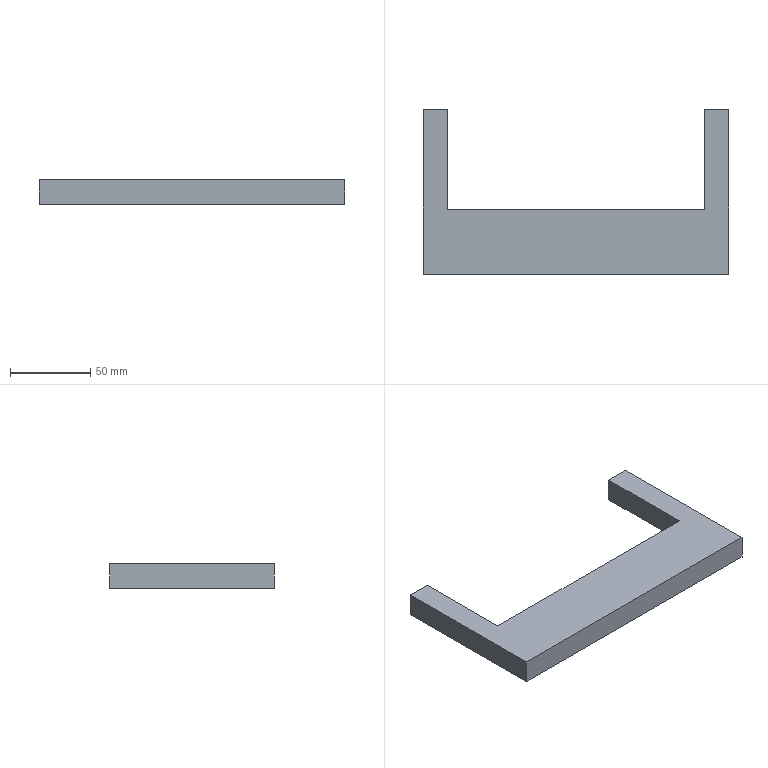Part | NX | features ejector support 2 | 1 solid | 10 faces | box 190 x 102.2 x 15 mm | volume 141990 mm3 | plane 10
STEP:
#1=CARTESIAN_POINT('',(-80.,40.,0.));
#2=VERTEX_POINT('',#1);
#3=CARTESIAN_POINT('',(-80.,102.2,0.));
#4=VERTEX_POINT('',#3);
#5=CARTESIAN_POINT('',(-80.,102.2,0.));
#6=DIRECTION('',(0.,-1.,0.));
#7=VECTOR('',#6,1000.);
#8=LINE('',#5,#7);
#9=EDGE_CURVE('',#2,#4,#8,.F.);
#10=ORIENTED_EDGE('',*,*,#9,.T.);
#11=CARTESIAN_POINT('',(-95.,102.2,0.));
#12=VERTEX_POINT('',#11);
#13=CARTESIAN_POINT('',(-95.,102.2,0.));
#14=DIRECTION('',(1.,0.,0.));
#15=VECTOR('',#14,1000.);
#16=LINE('',#13,#15);
#17=EDGE_CURVE('',#12,#4,#16,.T.);
#18=ORIENTED_EDGE('',*,*,#17,.F.);
#19=CARTESIAN_POINT('',(-95.,0.,0.));
#20=VERTEX_POINT('',#19);
#21=CARTESIAN_POINT('',(-95.,0.,0.));
#22=DIRECTION('',(0.,1.,0.));
#23=VECTOR('',#22,1000.);
#24=LINE('',#21,#23);
#25=EDGE_CURVE('',#20,#12,#24,.T.);
#26=ORIENTED_EDGE('',*,*,#25,.F.);
#27=CARTESIAN_POINT('',(95.,0.,0.));
#28=VERTEX_POINT('',#27);
#29=CARTESIAN_POINT('',(-95.,0.,0.));
#30=DIRECTION('',(1.,0.,0.));
#31=VECTOR('',#30,1000.);
#32=LINE('',#29,#31);
#33=EDGE_CURVE('',#28,#20,#32,.F.);
#34=ORIENTED_EDGE('',*,*,#33,.F.);
#35=CARTESIAN_POINT('',(95.,102.2,0.));
#36=VERTEX_POINT('',#35);
#37=CARTESIAN_POINT('',(95.,0.,0.));
#38=DIRECTION('',(0.,1.,0.));
#39=VECTOR('',#38,1000.);
#40=LINE('',#37,#39);
#41=EDGE_CURVE('',#36,#28,#40,.F.);
#42=ORIENTED_EDGE('',*,*,#41,.F.);
#43=CARTESIAN_POINT('',(80.,102.2,0.));
#44=VERTEX_POINT('',#43);
#45=CARTESIAN_POINT('',(-95.,102.2,0.));
#46=DIRECTION('',(1.,0.,0.));
#47=VECTOR('',#46,1000.);
#48=LINE('',#45,#47);
#49=EDGE_CURVE('',#44,#36,#48,.T.);
#50=ORIENTED_EDGE('',*,*,#49,.F.);
#51=CARTESIAN_POINT('',(80.,40.,0.));
#52=VERTEX_POINT('',#51);
#53=CARTESIAN_POINT('',(80.,102.2,0.));
#54=DIRECTION('',(0.,1.,0.));
#55=VECTOR('',#54,1000.);
#56=LINE('',#53,#55);
#57=EDGE_CURVE('',#44,#52,#56,.F.);
#58=ORIENTED_EDGE('',*,*,#57,.T.);
#59=CARTESIAN_POINT('',(-80.,40.,0.));
#60=DIRECTION('',(1.,0.,0.));
#61=VECTOR('',#60,1000.);
#62=LINE('',#59,#61);
#63=EDGE_CURVE('',#52,#2,#62,.F.);
#64=ORIENTED_EDGE('',*,*,#63,.T.);
#65=EDGE_LOOP('',(#10,#18,#26,#34,#42,#50,#58,#64));
#66=FACE_BOUND('',#65,.T.);
#67=CARTESIAN_POINT('',(95.,102.2,0.));
#68=DIRECTION('',(0.,0.,-1.));
#69=DIRECTION('',(-1.,0.,0.));
#70=AXIS2_PLACEMENT_3D('',#67,#68,#69);
#71=PLANE('',#70);
#72=ADVANCED_FACE('',(#66),#71,.F.);
#73=CARTESIAN_POINT('',(-80.,102.2,-15.));
#74=VERTEX_POINT('',#73);
#75=CARTESIAN_POINT('',(-80.,102.2,-15.));
#76=DIRECTION('',(0.,0.,1.));
#77=VECTOR('',#76,1000.);
#78=LINE('',#75,#77);
#79=EDGE_CURVE('',#4,#74,#78,.F.);
#80=ORIENTED_EDGE('',*,*,#79,.F.);
#81=ORIENTED_EDGE('',*,*,#9,.F.);
#82=CARTESIAN_POINT('',(-80.,40.,-15.));
#83=VERTEX_POINT('',#82);
#84=CARTESIAN_POINT('',(-80.,40.,0.));
#85=DIRECTION('',(0.,0.,1.));
#86=VECTOR('',#85,1000.);
#87=LINE('',#84,#86);
#88=EDGE_CURVE('',#2,#83,#87,.F.);
#89=ORIENTED_EDGE('',*,*,#88,.T.);
#90=CARTESIAN_POINT('',(-80.,102.2,-15.));
#91=DIRECTION('',(0.,1.,0.));
#92=VECTOR('',#91,1000.);
#93=LINE('',#90,#92);
#94=EDGE_CURVE('',#74,#83,#93,.F.);
#95=ORIENTED_EDGE('',*,*,#94,.F.);
#96=EDGE_LOOP('',(#80,#81,#89,#95));
#97=FACE_BOUND('',#96,.T.);
#98=CARTESIAN_POINT('',(-80.,102.2,0.));
#99=DIRECTION('',(-1.,0.,0.));
#100=DIRECTION('',(0.,-1.,0.));
#101=AXIS2_PLACEMENT_3D('',#98,#99,#100);
#102=PLANE('',#101);
#103=ADVANCED_FACE('',(#97),#102,.F.);
#104=ORIENTED_EDGE('',*,*,#88,.F.);
#105=ORIENTED_EDGE('',*,*,#63,.F.);
#106=CARTESIAN_POINT('',(80.,40.,-15.));
#107=VERTEX_POINT('',#106);
#108=CARTESIAN_POINT('',(80.,40.,0.));
#109=DIRECTION('',(0.,0.,-1.));
#110=VECTOR('',#109,1000.);
#111=LINE('',#108,#110);
#112=EDGE_CURVE('',#52,#107,#111,.T.);
#113=ORIENTED_EDGE('',*,*,#112,.T.);
#114=CARTESIAN_POINT('',(95.,40.,-15.));
#115=DIRECTION('',(-1.,0.,0.));
#116=VECTOR('',#115,1000.);
#117=LINE('',#114,#116);
#118=EDGE_CURVE('',#83,#107,#117,.F.);
#119=ORIENTED_EDGE('',*,*,#118,.F.);
#120=EDGE_LOOP('',(#104,#105,#113,#119));
#121=FACE_BOUND('',#120,.T.);
#122=CARTESIAN_POINT('',(-80.,40.,0.));
#123=DIRECTION('',(0.,-1.,0.));
#124=DIRECTION('',(1.,0.,0.));
#125=AXIS2_PLACEMENT_3D('',#122,#123,#124);
#126=PLANE('',#125);
#127=ADVANCED_FACE('',(#121),#126,.F.);
#128=ORIENTED_EDGE('',*,*,#112,.F.);
#129=ORIENTED_EDGE('',*,*,#57,.F.);
#130=CARTESIAN_POINT('',(80.,102.2,-15.));
#131=VERTEX_POINT('',#130);
#132=CARTESIAN_POINT('',(80.,102.2,-15.));
#133=DIRECTION('',(0.,0.,1.));
#134=VECTOR('',#133,1000.);
#135=LINE('',#132,#134);
#136=EDGE_CURVE('',#131,#44,#135,.T.);
#137=ORIENTED_EDGE('',*,*,#136,.F.);
#138=CARTESIAN_POINT('',(80.,102.2,-15.));
#139=DIRECTION('',(0.,1.,0.));
#140=VECTOR('',#139,1000.);
#141=LINE('',#138,#140);
#142=EDGE_CURVE('',#107,#131,#141,.T.);
#143=ORIENTED_EDGE('',*,*,#142,.F.);
#144=EDGE_LOOP('',(#128,#129,#137,#143));
#145=FACE_BOUND('',#144,.T.);
#146=CARTESIAN_POINT('',(80.,102.2,0.));
#147=DIRECTION('',(1.,0.,0.));
#148=DIRECTION('',(0.,0.,-1.));
#149=AXIS2_PLACEMENT_3D('',#146,#147,#148);
#150=PLANE('',#149);
#151=ADVANCED_FACE('',(#145),#150,.F.);
#152=CARTESIAN_POINT('',(95.,102.2,-15.));
#153=VERTEX_POINT('',#152);
#154=CARTESIAN_POINT('',(95.,102.2,-15.));
#155=DIRECTION('',(0.,0.,-1.));
#156=VECTOR('',#155,1000.);
#157=LINE('',#154,#156);
#158=EDGE_CURVE('',#153,#36,#157,.F.);
#159=ORIENTED_EDGE('',*,*,#158,.F.);
#160=CARTESIAN_POINT('',(95.,102.2,-15.));
#161=DIRECTION('',(-1.,0.,0.));
#162=VECTOR('',#161,1000.);
#163=LINE('',#160,#162);
#164=EDGE_CURVE('',#131,#153,#163,.F.);
#165=ORIENTED_EDGE('',*,*,#164,.F.);
#166=ORIENTED_EDGE('',*,*,#136,.T.);
#167=ORIENTED_EDGE('',*,*,#49,.T.);
#168=EDGE_LOOP('',(#159,#165,#166,#167));
#169=FACE_BOUND('',#168,.T.);
#170=CARTESIAN_POINT('',(-95.,102.2,-15.));
#171=DIRECTION('',(0.,1.,0.));
#172=DIRECTION('',(0.,0.,1.));
#173=AXIS2_PLACEMENT_3D('',#170,#171,#172);
#174=PLANE('',#173);
#175=ADVANCED_FACE('',(#169),#174,.T.);
#176=CARTESIAN_POINT('',(95.,0.,-15.));
#177=VERTEX_POINT('',#176);
#178=CARTESIAN_POINT('',(95.,102.2,-15.));
#179=DIRECTION('',(0.,1.,0.));
#180=VECTOR('',#179,1000.);
#181=LINE('',#178,#180);
#182=EDGE_CURVE('',#153,#177,#181,.F.);
#183=ORIENTED_EDGE('',*,*,#182,.F.);
#184=ORIENTED_EDGE('',*,*,#158,.T.);
#185=ORIENTED_EDGE('',*,*,#41,.T.);
#186=CARTESIAN_POINT('',(95.,0.,-15.));
#187=DIRECTION('',(0.,0.,-1.));
#188=VECTOR('',#187,1000.);
#189=LINE('',#186,#188);
#190=EDGE_CURVE('',#177,#28,#189,.F.);
#191=ORIENTED_EDGE('',*,*,#190,.F.);
#192=EDGE_LOOP('',(#183,#184,#185,#191));
#193=FACE_BOUND('',#192,.T.);
#194=CARTESIAN_POINT('',(95.,0.,-15.));
#195=DIRECTION('',(1.,0.,0.));
#196=DIRECTION('',(0.,0.,-1.));
#197=AXIS2_PLACEMENT_3D('',#194,#195,#196);
#198=PLANE('',#197);
#199=ADVANCED_FACE('',(#193),#198,.T.);
#200=CARTESIAN_POINT('',(-95.,0.,-15.));
#201=VERTEX_POINT('',#200);
#202=CARTESIAN_POINT('',(95.,0.,-15.));
#203=DIRECTION('',(-1.,0.,0.));
#204=VECTOR('',#203,1000.);
#205=LINE('',#202,#204);
#206=EDGE_CURVE('',#177,#201,#205,.T.);
#207=ORIENTED_EDGE('',*,*,#206,.F.);
#208=ORIENTED_EDGE('',*,*,#190,.T.);
#209=ORIENTED_EDGE('',*,*,#33,.T.);
#210=CARTESIAN_POINT('',(-95.,0.,-15.));
#211=DIRECTION('',(0.,0.,1.));
#212=VECTOR('',#211,1000.);
#213=LINE('',#210,#212);
#214=EDGE_CURVE('',#201,#20,#213,.T.);
#215=ORIENTED_EDGE('',*,*,#214,.F.);
#216=EDGE_LOOP('',(#207,#208,#209,#215));
#217=FACE_BOUND('',#216,.T.);
#218=CARTESIAN_POINT('',(-95.,0.,-15.));
#219=DIRECTION('',(0.,-1.,0.));
#220=DIRECTION('',(0.,0.,-1.));
#221=AXIS2_PLACEMENT_3D('',#218,#219,#220);
#222=PLANE('',#221);
#223=ADVANCED_FACE('',(#217),#222,.T.);
#224=CARTESIAN_POINT('',(-95.,102.2,-15.));
#225=VERTEX_POINT('',#224);
#226=CARTESIAN_POINT('',(-95.,102.2,-15.));
#227=DIRECTION('',(0.,1.,0.));
#228=VECTOR('',#227,1000.);
#229=LINE('',#226,#228);
#230=EDGE_CURVE('',#201,#225,#229,.T.);
#231=ORIENTED_EDGE('',*,*,#230,.F.);
#232=ORIENTED_EDGE('',*,*,#214,.T.);
#233=ORIENTED_EDGE('',*,*,#25,.T.);
#234=CARTESIAN_POINT('',(-95.,102.2,-15.));
#235=DIRECTION('',(0.,0.,1.));
#236=VECTOR('',#235,1000.);
#237=LINE('',#234,#236);
#238=EDGE_CURVE('',#225,#12,#237,.T.);
#239=ORIENTED_EDGE('',*,*,#238,.F.);
#240=EDGE_LOOP('',(#231,#232,#233,#239));
#241=FACE_BOUND('',#240,.T.);
#242=CARTESIAN_POINT('',(-95.,0.,-15.));
#243=DIRECTION('',(-1.,0.,0.));
#244=DIRECTION('',(0.,0.,1.));
#245=AXIS2_PLACEMENT_3D('',#242,#243,#244);
#246=PLANE('',#245);
#247=ADVANCED_FACE('',(#241),#246,.T.);
#248=ORIENTED_EDGE('',*,*,#238,.T.);
#249=ORIENTED_EDGE('',*,*,#17,.T.);
#250=ORIENTED_EDGE('',*,*,#79,.T.);
#251=CARTESIAN_POINT('',(95.,102.2,-15.));
#252=DIRECTION('',(-1.,0.,0.));
#253=VECTOR('',#252,1000.);
#254=LINE('',#251,#253);
#255=EDGE_CURVE('',#225,#74,#254,.F.);
#256=ORIENTED_EDGE('',*,*,#255,.F.);
#257=EDGE_LOOP('',(#248,#249,#250,#256));
#258=FACE_BOUND('',#257,.T.);
#259=CARTESIAN_POINT('',(-95.,102.2,-15.));
#260=DIRECTION('',(0.,1.,0.));
#261=DIRECTION('',(0.,0.,1.));
#262=AXIS2_PLACEMENT_3D('',#259,#260,#261);
#263=PLANE('',#262);
#264=ADVANCED_FACE('',(#258),#263,.T.);
#265=ORIENTED_EDGE('',*,*,#230,.T.);
#266=ORIENTED_EDGE('',*,*,#255,.T.);
#267=ORIENTED_EDGE('',*,*,#94,.T.);
#268=ORIENTED_EDGE('',*,*,#118,.T.);
#269=ORIENTED_EDGE('',*,*,#142,.T.);
#270=ORIENTED_EDGE('',*,*,#164,.T.);
#271=ORIENTED_EDGE('',*,*,#182,.T.);
#272=ORIENTED_EDGE('',*,*,#206,.T.);
#273=EDGE_LOOP('',(#265,#266,#267,#268,#269,#270,#271,#272));
#274=FACE_BOUND('',#273,.T.);
#275=CARTESIAN_POINT('',(95.,102.2,-15.));
#276=DIRECTION('',(0.,0.,-1.));
#277=DIRECTION('',(-1.,0.,0.));
#278=AXIS2_PLACEMENT_3D('',#275,#276,#277);
#279=PLANE('',#278);
#280=ADVANCED_FACE('',(#274),#279,.T.);
#281=CLOSED_SHELL('',(#72,#103,#127,#151,#175,#199,#223,#247,#264,#280));
#282=MANIFOLD_SOLID_BREP('',#281);
#283=(LENGTH_UNIT()NAMED_UNIT(*)SI_UNIT(.MILLI.,.METRE.));
#284=UNCERTAINTY_MEASURE_WITH_UNIT(LENGTH_MEASURE(0.00001),#283,'','');
#285=(NAMED_UNIT(*)PLANE_ANGLE_UNIT()SI_UNIT($,.RADIAN.));
#286=(NAMED_UNIT(*)SI_UNIT($,.STERADIAN.)SOLID_ANGLE_UNIT());
#287=(GEOMETRIC_REPRESENTATION_CONTEXT(3)GLOBAL_UNCERTAINTY_ASSIGNED_CONTEXT((#284))GLOBAL_UNIT_ASSIGNED_CONTEXT((#283,#285,#286))REPRESENTATION_CONTEXT('',''));
#288=ADVANCED_BREP_SHAPE_REPRESENTATION('',(#282),#287);